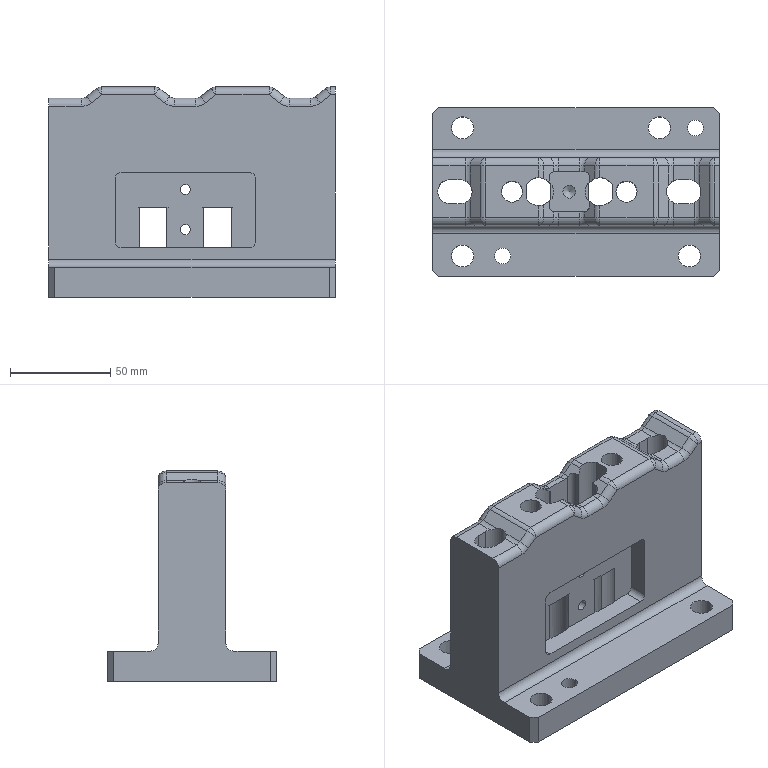Part | STEP file | 1_id282_x_t | 1 solid | 204 faces | box 143.3 x 84 x 105 mm | volume 430781 mm3 | cylinder 106 | plane 77 | sphere 10 | torus 10 | cone 1 | commonest cylinder face diameters 8 x41 6 x20 11 x8 16 x6 5.105 x4 7.938 x4